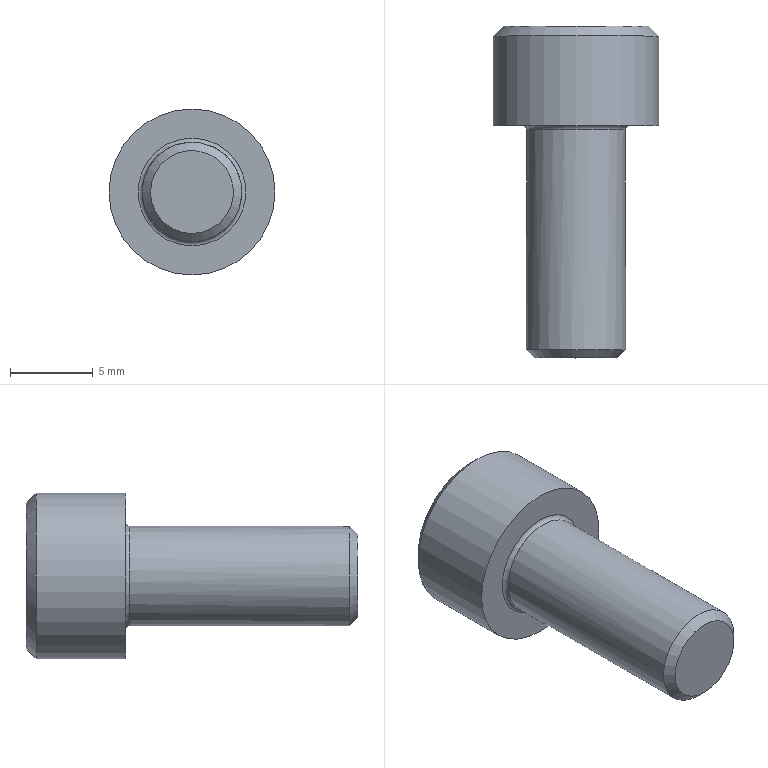Part | STEP file | solid 58 | 1 solid | 21 faces | box 10 x 20 x 10 mm | volume 794.444 mm3 | plane 10 | sphere 6 | cylinder 2 | cone 2 | torus 1 | commonest cylinder face diameters 6 x1 10 x1